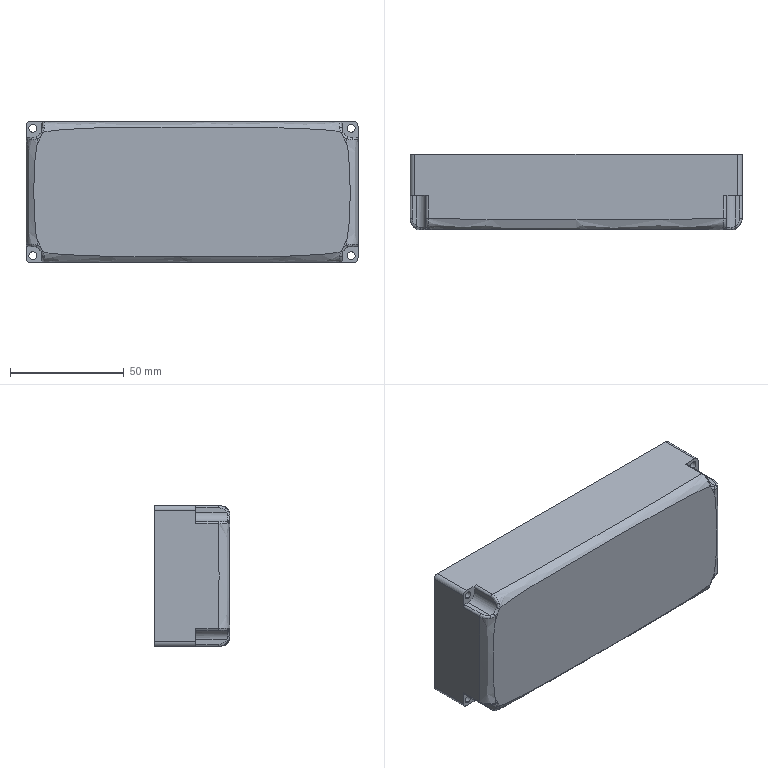Part | STEP file | 1 solid | 99 faces | volume 40401 mm3 | spline 36 | cylinder 36 | plane 27 | commonest cylinder face diameters 2 x8 3.4 x8 7.8 x6 11.4 x6 4 x4 8 x4